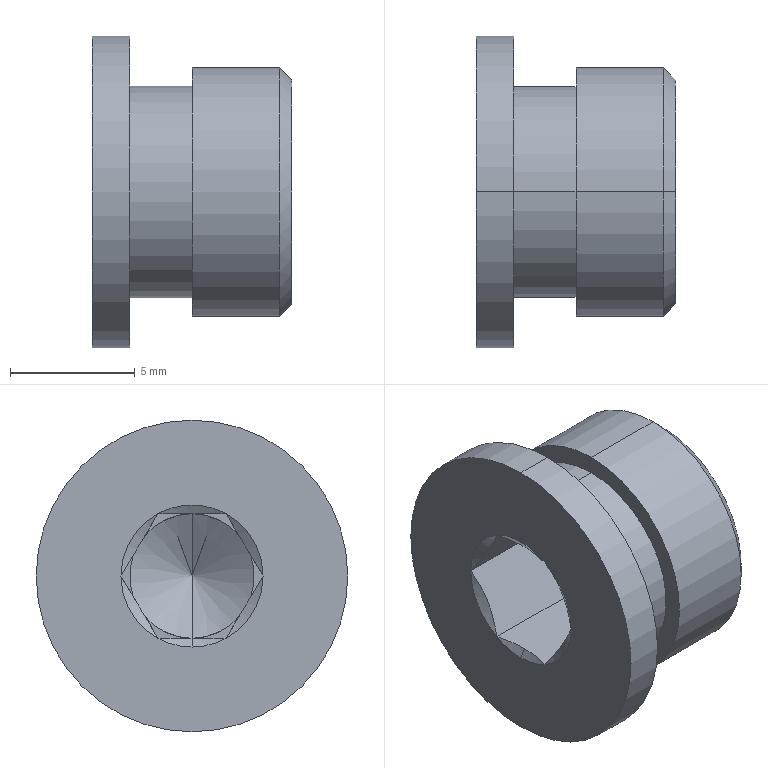Part | SolidWorks | features BaseBody 1 | 1 solid | 39 faces | box 8 x 12.5 x 12.5 mm | volume 511.919 mm3 | plane 20 | cone 11 | cylinder 8 | commonest cylinder face diameters 5 x2 8.5 x2 10 x2 12.5 x2
STEP:
#1=CARTESIAN_POINT('',(9.1,110.5,31.));
#2=VERTEX_POINT('',#1);
#3=CARTESIAN_POINT('',(9.1,110.5,22.));
#4=VERTEX_POINT('',#3);
#5=CARTESIAN_POINT('',(9.1,110.5,26.5));
#6=DIRECTION('',(1.,0.,0.));
#7=DIRECTION('',(0.,0.,1.));
#8=AXIS2_PLACEMENT_3D('',#5,#6,#7);
#9=CIRCLE('',#8,4.5);
#10=EDGE_CURVE('',#2,#4,#9,.T.);
#11=ORIENTED_EDGE('',*,*,#10,.F.);
#12=CARTESIAN_POINT('',(8.6,110.5,31.5));
#13=VERTEX_POINT('',#12);
#14=CARTESIAN_POINT('',(9.1,110.5,31.));
#15=DIRECTION('',(-0.7071,0.,0.7071));
#16=VECTOR('',#15,1000.);
#17=LINE('',#14,#16);
#18=EDGE_CURVE('',#2,#13,#17,.T.);
#19=ORIENTED_EDGE('',*,*,#18,.T.);
#20=CARTESIAN_POINT('',(8.6,110.5,21.5));
#21=VERTEX_POINT('',#20);
#22=CARTESIAN_POINT('',(8.6,110.5,26.5));
#23=DIRECTION('',(-1.,0.,0.));
#24=DIRECTION('',(0.,0.,1.));
#25=AXIS2_PLACEMENT_3D('',#22,#23,#24);
#26=CIRCLE('',#25,5.);
#27=EDGE_CURVE('',#21,#13,#26,.T.);
#28=ORIENTED_EDGE('',*,*,#27,.F.);
#29=CARTESIAN_POINT('',(9.1,110.5,22.));
#30=DIRECTION('',(-0.7071,0.,-0.7071));
#31=VECTOR('',#30,1000.);
#32=LINE('',#29,#31);
#33=EDGE_CURVE('',#4,#21,#32,.T.);
#34=ORIENTED_EDGE('',*,*,#33,.F.);
#35=EDGE_LOOP('',(#11,#19,#28,#34));
#36=FACE_OUTER_BOUND('',#35,.T.);
#37=CARTESIAN_POINT('',(9.1,110.5,26.5));
#38=DIRECTION('',(-1.,0.,0.));
#39=DIRECTION('',(0.,0.,-1.));
#40=AXIS2_PLACEMENT_3D('',#37,#38,#39);
#41=CONICAL_SURFACE('',#40,4.5,0.7854);
#42=ADVANCED_FACE('',(#36),#41,.T.);
#43=CARTESIAN_POINT('',(8.043,110.5,26.5));
#44=VERTEX_POINT('',#43);
#45=CARTESIAN_POINT('',(6.6,110.5,24.));
#46=VERTEX_POINT('',#45);
#47=CARTESIAN_POINT('',(6.6,110.5,24.));
#48=DIRECTION('',(-0.5,0.,-0.866));
#49=VECTOR('',#48,1000.);
#50=LINE('',#47,#49);
#51=EDGE_CURVE('',#44,#46,#50,.T.);
#52=ORIENTED_EDGE('',*,*,#51,.F.);
#53=CARTESIAN_POINT('',(6.6,110.5,29.));
#54=VERTEX_POINT('',#53);
#55=CARTESIAN_POINT('',(6.6,110.5,29.));
#56=DIRECTION('',(-0.5,0.,0.866));
#57=VECTOR('',#56,1000.);
#58=LINE('',#55,#57);
#59=EDGE_CURVE('',#44,#54,#58,.T.);
#60=ORIENTED_EDGE('',*,*,#59,.T.);
#61=CARTESIAN_POINT('',(6.6,110.5,26.5));
#62=DIRECTION('',(-1.,0.,0.));
#63=DIRECTION('',(0.,0.,-1.));
#64=AXIS2_PLACEMENT_3D('',#61,#62,#63);
#65=CIRCLE('',#64,2.5);
#66=EDGE_CURVE('',#54,#46,#65,.T.);
#67=ORIENTED_EDGE('',*,*,#66,.T.);
#68=EDGE_LOOP('',(#52,#60,#67));
#69=FACE_OUTER_BOUND('',#68,.T.);
#70=CARTESIAN_POINT('',(6.6,110.5,26.5));
#71=DIRECTION('',(-1.,0.,0.));
#72=DIRECTION('',(0.,0.,-1.));
#73=AXIS2_PLACEMENT_3D('',#70,#71,#72);
#74=CONICAL_SURFACE('',#73,2.5,1.047);
#75=ADVANCED_FACE('',(#69),#74,.F.);
#76=ORIENTED_EDGE('',*,*,#66,.F.);
#77=CARTESIAN_POINT('',(5.6,110.5,29.));
#78=VERTEX_POINT('',#77);
#79=CARTESIAN_POINT('',(22.671,110.5,29.));
#80=DIRECTION('',(-1.,0.,0.));
#81=VECTOR('',#80,1000.);
#82=LINE('',#79,#81);
#83=EDGE_CURVE('',#54,#78,#82,.T.);
#84=ORIENTED_EDGE('',*,*,#83,.T.);
#85=CARTESIAN_POINT('',(5.6,112.36,28.17));
#86=VERTEX_POINT('',#85);
#87=CARTESIAN_POINT('',(5.6,110.5,26.5));
#88=DIRECTION('',(1.,0.,0.));
#89=DIRECTION('',(0.,0.,1.));
#90=AXIS2_PLACEMENT_3D('',#87,#88,#89);
#91=CIRCLE('',#90,2.5);
#92=EDGE_CURVE('',#86,#78,#91,.T.);
#93=ORIENTED_EDGE('',*,*,#92,.F.);
#94=CARTESIAN_POINT('',(5.6,112.858,27.33));
#95=VERTEX_POINT('',#94);
#96=CARTESIAN_POINT('',(5.6,110.5,26.5));
#97=DIRECTION('',(-1.,0.,0.));
#98=DIRECTION('',(0.,0.,-1.));
#99=AXIS2_PLACEMENT_3D('',#96,#97,#98);
#100=CIRCLE('',#99,2.5);
#101=EDGE_CURVE('',#86,#95,#100,.T.);
#102=ORIENTED_EDGE('',*,*,#101,.T.);
#103=CARTESIAN_POINT('',(5.6,112.858,25.67));
#104=VERTEX_POINT('',#103);
#105=CARTESIAN_POINT('',(5.6,110.5,26.5));
#106=DIRECTION('',(1.,0.,0.));
#107=DIRECTION('',(0.,0.,1.));
#108=AXIS2_PLACEMENT_3D('',#105,#106,#107);
#109=CIRCLE('',#108,2.5);
#110=EDGE_CURVE('',#104,#95,#109,.T.);
#111=ORIENTED_EDGE('',*,*,#110,.F.);
#112=CARTESIAN_POINT('',(5.6,112.36,24.83));
#113=VERTEX_POINT('',#112);
#114=CARTESIAN_POINT('',(5.6,110.5,26.5));
#115=DIRECTION('',(-1.,0.,0.));
#116=DIRECTION('',(0.,0.,-1.));
#117=AXIS2_PLACEMENT_3D('',#114,#115,#116);
#118=CIRCLE('',#117,2.5);
#119=EDGE_CURVE('',#104,#113,#118,.T.);
#120=ORIENTED_EDGE('',*,*,#119,.T.);
#121=CARTESIAN_POINT('',(5.6,110.5,24.));
#122=VERTEX_POINT('',#121);
#123=CARTESIAN_POINT('',(5.6,110.5,26.5));
#124=DIRECTION('',(1.,0.,0.));
#125=DIRECTION('',(0.,0.,1.));
#126=AXIS2_PLACEMENT_3D('',#123,#124,#125);
#127=CIRCLE('',#126,2.5);
#128=EDGE_CURVE('',#122,#113,#127,.T.);
#129=ORIENTED_EDGE('',*,*,#128,.F.);
#130=CARTESIAN_POINT('',(22.671,110.5,24.));
#131=DIRECTION('',(-1.,0.,0.));
#132=VECTOR('',#131,1000.);
#133=LINE('',#130,#132);
#134=EDGE_CURVE('',#46,#122,#133,.T.);
#135=ORIENTED_EDGE('',*,*,#134,.F.);
#136=EDGE_LOOP('',(#76,#84,#93,#102,#111,#120,#129,#135));
#137=FACE_OUTER_BOUND('',#136,.T.);
#138=CARTESIAN_POINT('',(22.671,110.5,26.5));
#139=DIRECTION('',(-1.,0.,0.));
#140=DIRECTION('',(0.,0.,-1.));
#141=AXIS2_PLACEMENT_3D('',#138,#139,#140);
#142=CYLINDRICAL_SURFACE('',#141,2.5);
#143=ADVANCED_FACE('',(#137),#142,.F.);
#144=CARTESIAN_POINT('',(1.1,109.132,24.));
#145=VERTEX_POINT('',#144);
#146=CARTESIAN_POINT('',(1.302,110.5,24.));
#147=VERTEX_POINT('',#146);
#148=CARTESIAN_POINT('',(1.1,109.132,24.));
#149=CARTESIAN_POINT('',(1.161,109.353,24.));
#150=CARTESIAN_POINT('',(1.212,109.578,24.));
#151=CARTESIAN_POINT('',(1.283,110.036,24.));
#152=CARTESIAN_POINT('',(1.302,110.269,24.));
#153=CARTESIAN_POINT('',(1.302,110.5,24.));
#154=B_SPLINE_CURVE_WITH_KNOTS('',3,(#148,#149,#150,#151,#152,#153),.UNSPECIFIED.,.F.,.F.,(4,2,4),(0.001327,0.002017,0.002707),.UNSPECIFIED.);
#155=EDGE_CURVE('',#145,#147,#154,.T.);
#156=ORIENTED_EDGE('',*,*,#155,.T.);
#157=CARTESIAN_POINT('',(1.1,110.5,23.65));
#158=VERTEX_POINT('',#157);
#159=CARTESIAN_POINT('',(1.1,110.5,23.65));
#160=DIRECTION('',(-0.5,0.,-0.866));
#161=VECTOR('',#160,1000.);
#162=LINE('',#159,#161);
#163=EDGE_CURVE('',#147,#158,#162,.T.);
#164=ORIENTED_EDGE('',*,*,#163,.T.);
#165=CARTESIAN_POINT('',(1.1,110.5,26.5));
#166=DIRECTION('',(-1.,0.,0.));
#167=DIRECTION('',(0.,0.,-1.));
#168=AXIS2_PLACEMENT_3D('',#165,#166,#167);
#169=CIRCLE('',#168,2.85);
#170=EDGE_CURVE('',#158,#145,#169,.T.);
#171=ORIENTED_EDGE('',*,*,#170,.T.);
#172=EDGE_LOOP('',(#156,#164,#171));
#173=FACE_OUTER_BOUND('',#172,.T.);
#174=CARTESIAN_POINT('',(1.1,110.5,26.5));
#175=DIRECTION('',(-1.,0.,0.));
#176=DIRECTION('',(0.,0.,-1.));
#177=AXIS2_PLACEMENT_3D('',#174,#175,#176);
#178=CONICAL_SURFACE('',#177,2.85,1.047);
#179=ADVANCED_FACE('',(#173),#178,.F.);
#180=ORIENTED_EDGE('',*,*,#27,.T.);
#181=CARTESIAN_POINT('',(5.1,110.5,31.5));
#182=VERTEX_POINT('',#181);
#183=CARTESIAN_POINT('',(31.242,110.5,31.5));
#184=DIRECTION('',(-1.,0.,0.));
#185=VECTOR('',#184,1000.);
#186=LINE('',#183,#185);
#187=EDGE_CURVE('',#13,#182,#186,.T.);
#188=ORIENTED_EDGE('',*,*,#187,.T.);
#189=CARTESIAN_POINT('',(5.1,110.5,21.5));
#190=VERTEX_POINT('',#189);
#191=CARTESIAN_POINT('',(5.1,110.5,26.5));
#192=DIRECTION('',(1.,0.,0.));
#193=DIRECTION('',(0.,0.,1.));
#194=AXIS2_PLACEMENT_3D('',#191,#192,#193);
#195=CIRCLE('',#194,5.);
#196=EDGE_CURVE('',#182,#190,#195,.T.);
#197=ORIENTED_EDGE('',*,*,#196,.T.);
#198=CARTESIAN_POINT('',(31.242,110.5,21.5));
#199=DIRECTION('',(-1.,0.,0.));
#200=VECTOR('',#199,1000.);
#201=LINE('',#198,#200);
#202=EDGE_CURVE('',#21,#190,#201,.T.);
#203=ORIENTED_EDGE('',*,*,#202,.F.);
#204=EDGE_LOOP('',(#180,#188,#197,#203));
#205=FACE_OUTER_BOUND('',#204,.T.);
#206=CARTESIAN_POINT('',(31.242,110.5,26.5));
#207=DIRECTION('',(-1.,0.,0.));
#208=DIRECTION('',(0.,0.,-1.));
#209=AXIS2_PLACEMENT_3D('',#206,#207,#208);
#210=CYLINDRICAL_SURFACE('',#209,5.);
#211=ADVANCED_FACE('',(#205),#210,.T.);
#212=CARTESIAN_POINT('',(5.1,110.5,30.75));
#213=VERTEX_POINT('',#212);
#214=CARTESIAN_POINT('',(5.1,110.5,22.25));
#215=VERTEX_POINT('',#214);
#216=CARTESIAN_POINT('',(5.1,110.5,26.5));
#217=DIRECTION('',(1.,0.,0.));
#218=DIRECTION('',(0.,0.,1.));
#219=AXIS2_PLACEMENT_3D('',#216,#217,#218);
#220=CIRCLE('',#219,4.25);
#221=EDGE_CURVE('',#213,#215,#220,.T.);
#222=ORIENTED_EDGE('',*,*,#221,.F.);
#223=CARTESIAN_POINT('',(2.6,110.5,30.75));
#224=VERTEX_POINT('',#223);
#225=CARTESIAN_POINT('',(5.1,110.5,30.75));
#226=DIRECTION('',(-1.,0.,0.));
#227=VECTOR('',#226,1000.);
#228=LINE('',#225,#227);
#229=EDGE_CURVE('',#213,#224,#228,.T.);
#230=ORIENTED_EDGE('',*,*,#229,.T.);
#231=CARTESIAN_POINT('',(2.6,110.5,22.25));
#232=VERTEX_POINT('',#231);
#233=CARTESIAN_POINT('',(2.6,110.5,26.5));
#234=DIRECTION('',(1.,0.,0.));
#235=DIRECTION('',(0.,0.,1.));
#236=AXIS2_PLACEMENT_3D('',#233,#234,#235);
#237=CIRCLE('',#236,4.25);
#238=EDGE_CURVE('',#224,#232,#237,.T.);
#239=ORIENTED_EDGE('',*,*,#238,.T.);
#240=CARTESIAN_POINT('',(5.1,110.5,22.25));
#241=DIRECTION('',(-1.,0.,0.));
#242=VECTOR('',#241,1000.);
#243=LINE('',#240,#242);
#244=EDGE_CURVE('',#215,#232,#243,.T.);
#245=ORIENTED_EDGE('',*,*,#244,.F.);
#246=EDGE_LOOP('',(#222,#230,#239,#245));
#247=FACE_OUTER_BOUND('',#246,.T.);
#248=CARTESIAN_POINT('',(5.1,110.5,26.5));
#249=DIRECTION('',(-1.,0.,0.));
#250=DIRECTION('',(0.,0.,-1.));
#251=AXIS2_PLACEMENT_3D('',#248,#249,#250);
#252=CYLINDRICAL_SURFACE('',#251,4.25);
#253=ADVANCED_FACE('',(#247),#252,.T.);
#254=CARTESIAN_POINT('',(2.6,110.5,32.75));
#255=VERTEX_POINT('',#254);
#256=CARTESIAN_POINT('',(2.6,110.5,20.25));
#257=VERTEX_POINT('',#256);
#258=CARTESIAN_POINT('',(2.6,110.5,26.5));
#259=DIRECTION('',(1.,0.,0.));
#260=DIRECTION('',(0.,0.,1.));
#261=AXIS2_PLACEMENT_3D('',#258,#259,#260);
#262=CIRCLE('',#261,6.25);
#263=EDGE_CURVE('',#255,#257,#262,.T.);
#264=ORIENTED_EDGE('',*,*,#263,.F.);
#265=CARTESIAN_POINT('',(1.1,110.5,32.75));
#266=VERTEX_POINT('',#265);
#267=CARTESIAN_POINT('',(2.6,110.5,32.75));
#268=DIRECTION('',(-1.,0.,0.));
#269=VECTOR('',#268,1000.);
#270=LINE('',#267,#269);
#271=EDGE_CURVE('',#255,#266,#270,.T.);
#272=ORIENTED_EDGE('',*,*,#271,.T.);
#273=CARTESIAN_POINT('',(1.1,110.5,20.25));
#274=VERTEX_POINT('',#273);
#275=CARTESIAN_POINT('',(1.1,110.5,26.5));
#276=DIRECTION('',(1.,0.,0.));
#277=DIRECTION('',(0.,0.,1.));
#278=AXIS2_PLACEMENT_3D('',#275,#276,#277);
#279=CIRCLE('',#278,6.25);
#280=EDGE_CURVE('',#266,#274,#279,.T.);
#281=ORIENTED_EDGE('',*,*,#280,.T.);
#282=CARTESIAN_POINT('',(2.6,110.5,20.25));
#283=DIRECTION('',(-1.,0.,0.));
#284=VECTOR('',#283,1000.);
#285=LINE('',#282,#284);
#286=EDGE_CURVE('',#257,#274,#285,.T.);
#287=ORIENTED_EDGE('',*,*,#286,.F.);
#288=EDGE_LOOP('',(#264,#272,#281,#287));
#289=FACE_OUTER_BOUND('',#288,.T.);
#290=CARTESIAN_POINT('',(2.6,110.5,26.5));
#291=DIRECTION('',(-1.,0.,0.));
#292=DIRECTION('',(0.,0.,-1.));
#293=AXIS2_PLACEMENT_3D('',#290,#291,#292);
#294=CYLINDRICAL_SURFACE('',#293,6.25);
#295=ADVANCED_FACE('',(#289),#294,.T.);
#296=CARTESIAN_POINT('',(5.6,107.65,26.5));
#297=VERTEX_POINT('',#296);
#298=CARTESIAN_POINT('',(5.6,108.142,27.33));
#299=VERTEX_POINT('',#298);
#300=CARTESIAN_POINT('',(5.6,107.65,26.5));
#301=DIRECTION('',(0.,0.5098,0.8603));
#302=VECTOR('',#301,1000.);
#303=LINE('',#300,#302);
#304=EDGE_CURVE('',#297,#299,#303,.T.);
#305=ORIENTED_EDGE('',*,*,#304,.T.);
#306=CARTESIAN_POINT('',(5.6,108.142,25.67));
#307=VERTEX_POINT('',#306);
#308=CARTESIAN_POINT('',(5.6,110.5,26.5));
#309=DIRECTION('',(1.,0.,0.));
#310=DIRECTION('',(0.,0.,1.));
#311=AXIS2_PLACEMENT_3D('',#308,#309,#310);
#312=CIRCLE('',#311,2.5);
#313=EDGE_CURVE('',#299,#307,#312,.T.);
#314=ORIENTED_EDGE('',*,*,#313,.T.);
#315=CARTESIAN_POINT('',(5.6,107.65,26.5));
#316=DIRECTION('',(0.,-0.5098,0.8603));
#317=VECTOR('',#316,1000.);
#318=LINE('',#315,#317);
#319=EDGE_CURVE('',#307,#297,#318,.T.);
#320=ORIENTED_EDGE('',*,*,#319,.T.);
#321=EDGE_LOOP('',(#305,#314,#320));
#322=FACE_OUTER_BOUND('',#321,.T.);
#323=CARTESIAN_POINT('',(5.6,110.5,31.309));
#324=DIRECTION('',(1.,0.,0.));
#325=DIRECTION('',(0.,0.,1.));
#326=AXIS2_PLACEMENT_3D('',#323,#324,#325);
#327=PLANE('',#326);
#328=ADVANCED_FACE('',(#322),#327,.F.);
#329=CARTESIAN_POINT('',(5.6,109.132,24.));
#330=VERTEX_POINT('',#329);
#331=CARTESIAN_POINT('',(5.6,108.64,24.83));
#332=VERTEX_POINT('',#331);
#333=CARTESIAN_POINT('',(5.6,107.65,26.5));
#334=DIRECTION('',(0.,-0.5098,0.8603));
#335=VECTOR('',#334,1000.);
#336=LINE('',#333,#335);
#337=EDGE_CURVE('',#330,#332,#336,.T.);
#338=ORIENTED_EDGE('',*,*,#337,.T.);
#339=CARTESIAN_POINT('',(5.6,110.5,26.5));
#340=DIRECTION('',(-1.,0.,0.));
#341=DIRECTION('',(0.,0.,-1.));
#342=AXIS2_PLACEMENT_3D('',#339,#340,#341);
#343=CIRCLE('',#342,2.5);
#344=EDGE_CURVE('',#122,#332,#343,.T.);
#345=ORIENTED_EDGE('',*,*,#344,.F.);
#346=CARTESIAN_POINT('',(5.6,109.132,24.));
#347=DIRECTION('',(0.,-1.,0.));
#348=VECTOR('',#347,1000.);
#349=LINE('',#346,#348);
#350=EDGE_CURVE('',#122,#330,#349,.T.);
#351=ORIENTED_EDGE('',*,*,#350,.T.);
#352=EDGE_LOOP('',(#338,#345,#351));
#353=FACE_OUTER_BOUND('',#352,.T.);
#354=CARTESIAN_POINT('',(5.6,110.5,31.309));
#355=DIRECTION('',(1.,0.,0.));
#356=DIRECTION('',(0.,0.,1.));
#357=AXIS2_PLACEMENT_3D('',#354,#355,#356);
#358=PLANE('',#357);
#359=ADVANCED_FACE('',(#353),#358,.F.);
#360=CARTESIAN_POINT('',(5.6,111.868,24.));
#361=VERTEX_POINT('',#360);
#362=CARTESIAN_POINT('',(5.6,109.132,24.));
#363=DIRECTION('',(0.,-1.,0.));
#364=VECTOR('',#363,1000.);
#365=LINE('',#362,#364);
#366=EDGE_CURVE('',#361,#122,#365,.T.);
#367=ORIENTED_EDGE('',*,*,#366,.T.);
#368=ORIENTED_EDGE('',*,*,#128,.T.);
#369=CARTESIAN_POINT('',(5.6,113.35,26.5));
#370=DIRECTION('',(0.,-0.5098,-0.8603));
#371=VECTOR('',#370,1000.);
#372=LINE('',#369,#371);
#373=EDGE_CURVE('',#113,#361,#372,.T.);
#374=ORIENTED_EDGE('',*,*,#373,.T.);
#375=EDGE_LOOP('',(#367,#368,#374));
#376=FACE_OUTER_BOUND('',#375,.T.);
#377=CARTESIAN_POINT('',(5.6,110.5,31.309));
#378=DIRECTION('',(1.,0.,0.));
#379=DIRECTION('',(0.,0.,1.));
#380=AXIS2_PLACEMENT_3D('',#377,#378,#379);
#381=PLANE('',#380);
#382=ADVANCED_FACE('',(#376),#381,.F.);
#383=CARTESIAN_POINT('',(5.6,113.35,26.5));
#384=VERTEX_POINT('',#383);
#385=CARTESIAN_POINT('',(5.6,113.35,26.5));
#386=DIRECTION('',(0.,-0.5098,-0.8603));
#387=VECTOR('',#386,1000.);
#388=LINE('',#385,#387);
#389=EDGE_CURVE('',#384,#104,#388,.T.);
#390=ORIENTED_EDGE('',*,*,#389,.T.);
#391=ORIENTED_EDGE('',*,*,#110,.T.);
#392=CARTESIAN_POINT('',(5.6,113.35,26.5));
#393=DIRECTION('',(0.,0.5098,-0.8603));
#394=VECTOR('',#393,1000.);
#395=LINE('',#392,#394);
#396=EDGE_CURVE('',#95,#384,#395,.T.);
#397=ORIENTED_EDGE('',*,*,#396,.T.);
#398=EDGE_LOOP('',(#390,#391,#397));
#399=FACE_OUTER_BOUND('',#398,.T.);
#400=CARTESIAN_POINT('',(5.6,110.5,31.309));
#401=DIRECTION('',(1.,0.,0.));
#402=DIRECTION('',(0.,0.,1.));
#403=AXIS2_PLACEMENT_3D('',#400,#401,#402);
#404=PLANE('',#403);
#405=ADVANCED_FACE('',(#399),#404,.F.);
#406=CARTESIAN_POINT('',(5.6,109.132,29.));
#407=VERTEX_POINT('',#406);
#408=CARTESIAN_POINT('',(5.6,109.132,29.));
#409=DIRECTION('',(0.,1.,0.));
#410=VECTOR('',#409,1000.);
#411=LINE('',#408,#410);
#412=EDGE_CURVE('',#407,#78,#411,.T.);
#413=ORIENTED_EDGE('',*,*,#412,.T.);
#414=CARTESIAN_POINT('',(5.6,108.64,28.17));
#415=VERTEX_POINT('',#414);
#416=CARTESIAN_POINT('',(5.6,110.5,26.5));
#417=DIRECTION('',(1.,0.,0.));
#418=DIRECTION('',(0.,0.,1.));
#419=AXIS2_PLACEMENT_3D('',#416,#417,#418);
#420=CIRCLE('',#419,2.5);
#421=EDGE_CURVE('',#78,#415,#420,.T.);
#422=ORIENTED_EDGE('',*,*,#421,.T.);
#423=CARTESIAN_POINT('',(5.6,107.65,26.5));
#424=DIRECTION('',(0.,0.5098,0.8603));
#425=VECTOR('',#424,1000.);
#426=LINE('',#423,#425);
#427=EDGE_CURVE('',#415,#407,#426,.T.);
#428=ORIENTED_EDGE('',*,*,#427,.T.);
#429=EDGE_LOOP('',(#413,#422,#428));
#430=FACE_OUTER_BOUND('',#429,.T.);
#431=CARTESIAN_POINT('',(5.6,110.5,31.309));
#432=DIRECTION('',(1.,0.,0.));
#433=DIRECTION('',(0.,0.,1.));
#434=AXIS2_PLACEMENT_3D('',#431,#432,#433);
#435=PLANE('',#434);
#436=ADVANCED_FACE('',(#430),#435,.F.);
#437=CARTESIAN_POINT('',(2.6,110.5,26.5));
#438=DIRECTION('',(1.,0.,0.));
#439=DIRECTION('',(0.,0.,1.));
#440=AXIS2_PLACEMENT_3D('',#437,#438,#439);
#441=CIRCLE('',#440,6.25);
#442=EDGE_CURVE('',#257,#255,#441,.T.);
#443=ORIENTED_EDGE('',*,*,#442,.T.);
#444=ORIENTED_EDGE('',*,*,#263,.T.);
#445=EDGE_LOOP('',(#443,#444));
#446=FACE_OUTER_BOUND('',#445,.T.);
#447=CARTESIAN_POINT('',(2.6,110.5,26.5));
#448=DIRECTION('',(1.,0.,0.));
#449=DIRECTION('',(0.,0.,1.));
#450=AXIS2_PLACEMENT_3D('',#447,#448,#449);
#451=CIRCLE('',#450,4.25);
#452=EDGE_CURVE('',#232,#224,#451,.T.);
#453=ORIENTED_EDGE('',*,*,#452,.F.);
#454=ORIENTED_EDGE('',*,*,#238,.F.);
#455=EDGE_LOOP('',(#453,#454));
#456=FACE_BOUND('',#455,.T.);
#457=CARTESIAN_POINT('',(2.6,110.5,26.5));
#458=DIRECTION('',(1.,0.,0.));
#459=DIRECTION('',(0.,0.,1.));
#460=AXIS2_PLACEMENT_3D('',#457,#458,#459);
#461=PLANE('',#460);
#462=ADVANCED_FACE('',(#446,#456),#461,.T.);
#463=ORIENTED_EDGE('',*,*,#271,.F.);
#464=ORIENTED_EDGE('',*,*,#442,.F.);
#465=ORIENTED_EDGE('',*,*,#286,.T.);
#466=CARTESIAN_POINT('',(1.1,110.5,26.5));
#467=DIRECTION('',(1.,0.,0.));
#468=DIRECTION('',(0.,0.,1.));
#469=AXIS2_PLACEMENT_3D('',#466,#467,#468);
#470=CIRCLE('',#469,6.25);
#471=EDGE_CURVE('',#274,#266,#470,.T.);
#472=ORIENTED_EDGE('',*,*,#471,.T.);
#473=EDGE_LOOP('',(#463,#464,#465,#472));
#474=FACE_OUTER_BOUND('',#473,.T.);
#475=CARTESIAN_POINT('',(2.6,110.5,26.5));
#476=DIRECTION('',(-1.,0.,0.));
#477=DIRECTION('',(0.,0.,-1.));
#478=AXIS2_PLACEMENT_3D('',#475,#476,#477);
#479=CYLINDRICAL_SURFACE('',#478,6.25);
#480=ADVANCED_FACE('',(#474),#479,.T.);
#481=CARTESIAN_POINT('',(1.1,109.132,29.));
#482=VERTEX_POINT('',#481);
#483=CARTESIAN_POINT('',(1.1,111.868,29.));
#484=VERTEX_POINT('',#483);
#485=CARTESIAN_POINT('',(1.1,110.5,26.5));
#486=DIRECTION('',(-1.,0.,0.));
#487=DIRECTION('',(0.,0.,-1.));
#488=AXIS2_PLACEMENT_3D('',#485,#486,#487);
#489=CIRCLE('',#488,2.85);
#490=EDGE_CURVE('',#482,#484,#489,.T.);
#491=ORIENTED_EDGE('',*,*,#490,.F.);
#492=CARTESIAN_POINT('',(1.1,107.65,26.5));
#493=VERTEX_POINT('',#492);
#494=CARTESIAN_POINT('',(1.1,110.5,26.5));
#495=DIRECTION('',(-1.,0.,0.));
#496=DIRECTION('',(0.,0.,-1.));
#497=AXIS2_PLACEMENT_3D('',#494,#495,#496);
#498=CIRCLE('',#497,2.85);
#499=EDGE_CURVE('',#493,#482,#498,.T.);
#500=ORIENTED_EDGE('',*,*,#499,.F.);
#501=CARTESIAN_POINT('',(1.1,110.5,26.5));
#502=DIRECTION('',(-1.,0.,0.));
#503=DIRECTION('',(0.,0.,-1.));
#504=AXIS2_PLACEMENT_3D('',#501,#502,#503);
#505=CIRCLE('',#504,2.85);
#506=EDGE_CURVE('',#145,#493,#505,.T.);
#507=ORIENTED_EDGE('',*,*,#506,.F.);
#508=ORIENTED_EDGE('',*,*,#170,.F.);
#509=CARTESIAN_POINT('',(1.1,111.868,24.));
#510=VERTEX_POINT('',#509);
#511=CARTESIAN_POINT('',(1.1,110.5,26.5));
#512=DIRECTION('',(-1.,0.,0.));
#513=DIRECTION('',(0.,0.,-1.));
#514=AXIS2_PLACEMENT_3D('',#511,#512,#513);
#515=CIRCLE('',#514,2.85);
#516=EDGE_CURVE('',#510,#158,#515,.T.);
#517=ORIENTED_EDGE('',*,*,#516,.F.);
#518=CARTESIAN_POINT('',(1.1,113.35,26.5));
#519=VERTEX_POINT('',#518);
#520=CARTESIAN_POINT('',(1.1,110.5,26.5));
#521=DIRECTION('',(-1.,0.,0.));
#522=DIRECTION('',(0.,0.,-1.));
#523=AXIS2_PLACEMENT_3D('',#520,#521,#522);
#524=CIRCLE('',#523,2.85);
#525=EDGE_CURVE('',#519,#510,#524,.T.);
#526=ORIENTED_EDGE('',*,*,#525,.F.);
#527=CARTESIAN_POINT('',(1.1,110.5,26.5));
#528=DIRECTION('',(-1.,0.,0.));
#529=DIRECTION('',(0.,0.,-1.));
#530=AXIS2_PLACEMENT_3D('',#527,#528,#529);
#531=CIRCLE('',#530,2.85);
#532=EDGE_CURVE('',#484,#519,#531,.T.);
#533=ORIENTED_EDGE('',*,*,#532,.F.);
#534=EDGE_LOOP('',(#491,#500,#507,#508,#517,#526,#533));
#535=FACE_BOUND('',#534,.T.);
#536=ORIENTED_EDGE('',*,*,#471,.F.);
#537=ORIENTED_EDGE('',*,*,#280,.F.);
#538=EDGE_LOOP('',(#536,#537));
#539=FACE_OUTER_BOUND('',#538,.T.);
#540=CARTESIAN_POINT('',(1.1,110.5,26.5));
#541=DIRECTION('',(1.,0.,0.));
#542=DIRECTION('',(0.,0.,1.));
#543=AXIS2_PLACEMENT_3D('',#540,#541,#542);
#544=PLANE('',#543);
#545=ADVANCED_FACE('',(#535,#539),#544,.F.);
#546=ORIENTED_EDGE('',*,*,#229,.F.);
#547=CARTESIAN_POINT('',(5.1,110.5,26.5));
#548=DIRECTION('',(1.,0.,0.));
#549=DIRECTION('',(0.,0.,1.));
#550=AXIS2_PLACEMENT_3D('',#547,#548,#549);
#551=CIRCLE('',#550,4.25);
#552=EDGE_CURVE('',#215,#213,#551,.T.);
#553=ORIENTED_EDGE('',*,*,#552,.F.);
#554=ORIENTED_EDGE('',*,*,#244,.T.);
#555=ORIENTED_EDGE('',*,*,#452,.T.);
#556=EDGE_LOOP('',(#546,#553,#554,#555));
#557=FACE_OUTER_BOUND('',#556,.T.);
#558=CARTESIAN_POINT('',(5.1,110.5,26.5));
#559=DIRECTION('',(-1.,0.,0.));
#560=DIRECTION('',(0.,0.,-1.));
#561=AXIS2_PLACEMENT_3D('',#558,#559,#560);
#562=CYLINDRICAL_SURFACE('',#561,4.25);
#563=ADVANCED_FACE('',(#557),#562,.T.);
#564=CARTESIAN_POINT('',(5.1,110.5,26.5));
#565=DIRECTION('',(1.,0.,0.));
#566=DIRECTION('',(0.,0.,1.));
#567=AXIS2_PLACEMENT_3D('',#564,#565,#566);
#568=CIRCLE('',#567,5.);
#569=EDGE_CURVE('',#190,#182,#568,.T.);
#570=ORIENTED_EDGE('',*,*,#569,.F.);
#571=ORIENTED_EDGE('',*,*,#196,.F.);
#572=EDGE_LOOP('',(#570,#571));
#573=FACE_OUTER_BOUND('',#572,.T.);
#574=ORIENTED_EDGE('',*,*,#552,.T.);
#575=ORIENTED_EDGE('',*,*,#221,.T.);
#576=EDGE_LOOP('',(#574,#575));
#577=FACE_BOUND('',#576,.T.);
#578=CARTESIAN_POINT('',(5.1,110.5,26.5));
#579=DIRECTION('',(1.,0.,0.));
#580=DIRECTION('',(0.,0.,1.));
#581=AXIS2_PLACEMENT_3D('',#578,#579,#580);
#582=PLANE('',#581);
#583=ADVANCED_FACE('',(#573,#577),#582,.F.);
#584=ORIENTED_EDGE('',*,*,#187,.F.);
#585=CARTESIAN_POINT('',(8.6,110.5,26.5));
#586=DIRECTION('',(-1.,0.,0.));
#587=DIRECTION('',(0.,0.,1.));
#588=AXIS2_PLACEMENT_3D('',#585,#586,#587);
#589=CIRCLE('',#588,5.);
#590=EDGE_CURVE('',#13,#21,#589,.T.);
#591=ORIENTED_EDGE('',*,*,#590,.T.);
#592=ORIENTED_EDGE('',*,*,#202,.T.);
#593=ORIENTED_EDGE('',*,*,#569,.T.);
#594=EDGE_LOOP('',(#584,#591,#592,#593));
#595=FACE_OUTER_BOUND('',#594,.T.);
#596=CARTESIAN_POINT('',(31.242,110.5,26.5));
#597=DIRECTION('',(-1.,0.,0.));
#598=DIRECTION('',(0.,0.,-1.));
#599=AXIS2_PLACEMENT_3D('',#596,#597,#598);
#600=CYLINDRICAL_SURFACE('',#599,5.);
#601=ADVANCED_FACE('',(#595),#600,.T.);
#602=CARTESIAN_POINT('',(9.1,110.5,26.5));
#603=DIRECTION('',(1.,0.,0.));
#604=DIRECTION('',(0.,0.,1.));
#605=AXIS2_PLACEMENT_3D('',#602,#603,#604);
#606=CIRCLE('',#605,4.5);
#607=EDGE_CURVE('',#4,#2,#606,.T.);
#608=ORIENTED_EDGE('',*,*,#607,.T.);
#609=ORIENTED_EDGE('',*,*,#10,.T.);
#610=EDGE_LOOP('',(#608,#609));
#611=FACE_OUTER_BOUND('',#610,.T.);
#612=CARTESIAN_POINT('',(9.1,110.5,26.5));
#613=DIRECTION('',(1.,0.,0.));
#614=DIRECTION('',(0.,0.,1.));
#615=AXIS2_PLACEMENT_3D('',#612,#613,#614);
#616=PLANE('',#615);
#617=ADVANCED_FACE('',(#611),#616,.T.);
#618=CARTESIAN_POINT('',(5.6,107.65,26.5));
#619=DIRECTION('',(-1.,0.,0.));
#620=VECTOR('',#619,1000.);
#621=LINE('',#618,#620);
#622=EDGE_CURVE('',#297,#493,#621,.T.);
#623=ORIENTED_EDGE('',*,*,#622,.T.);
#624=CARTESIAN_POINT('',(1.1,109.132,29.));
#625=CARTESIAN_POINT('',(1.24,108.89,28.592));
#626=CARTESIAN_POINT('',(1.33,108.644,28.178));
#627=CARTESIAN_POINT('',(1.33,108.266,27.539));
#628=CARTESIAN_POINT('',(1.308,108.14,27.327));
#629=CARTESIAN_POINT('',(1.228,107.893,26.91));
#630=CARTESIAN_POINT('',(1.17,107.771,26.704));
#631=CARTESIAN_POINT('',(1.1,107.65,26.5));
#632=B_SPLINE_CURVE_WITH_KNOTS('',3,(#624,#625,#626,#627,#628,#629,#630,#631),.UNSPECIFIED.,.F.,.F.,(4,2,2,4),(0.00000024,0.001469,0.002204,0.002938),.UNSPECIFIED.);
#633=EDGE_CURVE('',#482,#493,#632,.T.);
#634=ORIENTED_EDGE('',*,*,#633,.F.);
#635=CARTESIAN_POINT('',(5.6,109.132,29.));
#636=DIRECTION('',(-1.,0.,0.));
#637=VECTOR('',#636,1000.);
#638=LINE('',#635,#637);
#639=EDGE_CURVE('',#407,#482,#638,.T.);
#640=ORIENTED_EDGE('',*,*,#639,.F.);
#641=ORIENTED_EDGE('',*,*,#427,.F.);
#642=CARTESIAN_POINT('',(5.6,107.65,26.5));
#643=DIRECTION('',(0.,0.5098,0.8603));
#644=VECTOR('',#643,1000.);
#645=LINE('',#642,#644);
#646=EDGE_CURVE('',#299,#415,#645,.T.);
#647=ORIENTED_EDGE('',*,*,#646,.F.);
#648=ORIENTED_EDGE('',*,*,#304,.F.);
#649=EDGE_LOOP('',(#623,#634,#640,#641,#647,#648));
#650=FACE_OUTER_BOUND('',#649,.T.);
#651=CARTESIAN_POINT('',(5.6,107.65,26.5));
#652=DIRECTION('',(0.,-0.8603,0.5098));
#653=DIRECTION('',(0.,-0.5098,-0.8603));
#654=AXIS2_PLACEMENT_3D('',#651,#652,#653);
#655=PLANE('',#654);
#656=ADVANCED_FACE('',(#650),#655,.F.);
#657=CARTESIAN_POINT('',(5.6,109.132,24.));
#658=DIRECTION('',(-1.,0.,0.));
#659=VECTOR('',#658,1000.);
#660=LINE('',#657,#659);
#661=EDGE_CURVE('',#330,#145,#660,.T.);
#662=ORIENTED_EDGE('',*,*,#661,.T.);
#663=CARTESIAN_POINT('',(1.1,107.65,26.5));
#664=CARTESIAN_POINT('',(1.24,107.892,26.092));
#665=CARTESIAN_POINT('',(1.33,108.137,25.678));
#666=CARTESIAN_POINT('',(1.33,108.516,25.039));
#667=CARTESIAN_POINT('',(1.308,108.642,24.827));
#668=CARTESIAN_POINT('',(1.228,108.889,24.41));
#669=CARTESIAN_POINT('',(1.17,109.011,24.204));
#670=CARTESIAN_POINT('',(1.1,109.132,24.));
#671=B_SPLINE_CURVE_WITH_KNOTS('',3,(#663,#664,#665,#666,#667,#668,#669,#670),.UNSPECIFIED.,.F.,.F.,(4,2,2,4),(0.00000024,0.001469,0.002204,0.002938),.UNSPECIFIED.);
#672=EDGE_CURVE('',#493,#145,#671,.T.);
#673=ORIENTED_EDGE('',*,*,#672,.F.);
#674=ORIENTED_EDGE('',*,*,#622,.F.);
#675=ORIENTED_EDGE('',*,*,#319,.F.);
#676=CARTESIAN_POINT('',(5.6,107.65,26.5));
#677=DIRECTION('',(0.,-0.5098,0.8603));
#678=VECTOR('',#677,1000.);
#679=LINE('',#676,#678);
#680=EDGE_CURVE('',#332,#307,#679,.T.);
#681=ORIENTED_EDGE('',*,*,#680,.F.);
#682=ORIENTED_EDGE('',*,*,#337,.F.);
#683=EDGE_LOOP('',(#662,#673,#674,#675,#681,#682));
#684=FACE_OUTER_BOUND('',#683,.T.);
#685=CARTESIAN_POINT('',(5.6,107.65,26.5));
#686=DIRECTION('',(0.,-0.8603,-0.5098));
#687=DIRECTION('',(0.,0.5098,-0.8603));
#688=AXIS2_PLACEMENT_3D('',#685,#686,#687);
#689=PLANE('',#688);
#690=ADVANCED_FACE('',(#684),#689,.F.);
#691=CARTESIAN_POINT('',(5.6,111.868,24.));
#692=DIRECTION('',(-1.,0.,0.));
#693=VECTOR('',#692,1000.);
#694=LINE('',#691,#693);
#695=EDGE_CURVE('',#361,#510,#694,.T.);
#696=ORIENTED_EDGE('',*,*,#695,.T.);
#697=CARTESIAN_POINT('',(1.302,110.5,24.));
#698=CARTESIAN_POINT('',(1.302,110.731,24.));
#699=CARTESIAN_POINT('',(1.283,110.96,24.));
#700=CARTESIAN_POINT('',(1.213,111.418,24.));
#701=CARTESIAN_POINT('',(1.162,111.646,24.));
#702=CARTESIAN_POINT('',(1.1,111.868,24.));
#703=B_SPLINE_CURVE_WITH_KNOTS('',3,(#697,#698,#699,#700,#701,#702),.UNSPECIFIED.,.F.,.F.,(4,2,4),(0.002707,0.003396,0.004086),.UNSPECIFIED.);
#704=EDGE_CURVE('',#147,#510,#703,.T.);
#705=ORIENTED_EDGE('',*,*,#704,.F.);
#706=ORIENTED_EDGE('',*,*,#155,.F.);
#707=ORIENTED_EDGE('',*,*,#661,.F.);
#708=ORIENTED_EDGE('',*,*,#350,.F.);
#709=ORIENTED_EDGE('',*,*,#366,.F.);
#710=EDGE_LOOP('',(#696,#705,#706,#707,#708,#709));
#711=FACE_OUTER_BOUND('',#710,.T.);
#712=CARTESIAN_POINT('',(5.6,109.132,24.));
#713=DIRECTION('',(0.,0.,-1.));
#714=DIRECTION('',(1.,0.,0.));
#715=AXIS2_PLACEMENT_3D('',#712,#713,#714);
#716=PLANE('',#715);
#717=ADVANCED_FACE('',(#711),#716,.F.);
#718=CARTESIAN_POINT('',(5.6,113.35,26.5));
#719=DIRECTION('',(-1.,0.,0.));
#720=VECTOR('',#719,1000.);
#721=LINE('',#718,#720);
#722=EDGE_CURVE('',#384,#519,#721,.T.);
#723=ORIENTED_EDGE('',*,*,#722,.T.);
#724=CARTESIAN_POINT('',(1.1,111.868,24.));
#725=CARTESIAN_POINT('',(1.24,112.11,24.408));
#726=CARTESIAN_POINT('',(1.33,112.356,24.822));
#727=CARTESIAN_POINT('',(1.33,112.734,25.461));
#728=CARTESIAN_POINT('',(1.308,112.86,25.673));
#729=CARTESIAN_POINT('',(1.228,113.107,26.09));
#730=CARTESIAN_POINT('',(1.17,113.229,26.296));
#731=CARTESIAN_POINT('',(1.1,113.35,26.5));
#732=B_SPLINE_CURVE_WITH_KNOTS('',3,(#724,#725,#726,#727,#728,#729,#730,#731),.UNSPECIFIED.,.F.,.F.,(4,2,2,4),(0.00000024,0.001469,0.002204,0.002938),.UNSPECIFIED.);
#733=EDGE_CURVE('',#510,#519,#732,.T.);
#734=ORIENTED_EDGE('',*,*,#733,.F.);
#735=ORIENTED_EDGE('',*,*,#695,.F.);
#736=ORIENTED_EDGE('',*,*,#373,.F.);
#737=CARTESIAN_POINT('',(5.6,113.35,26.5));
#738=DIRECTION('',(0.,-0.5098,-0.8603));
#739=VECTOR('',#738,1000.);
#740=LINE('',#737,#739);
#741=EDGE_CURVE('',#104,#113,#740,.T.);
#742=ORIENTED_EDGE('',*,*,#741,.F.);
#743=ORIENTED_EDGE('',*,*,#389,.F.);
#744=EDGE_LOOP('',(#723,#734,#735,#736,#742,#743));
#745=FACE_OUTER_BOUND('',#744,.T.);
#746=CARTESIAN_POINT('',(5.6,113.35,26.5));
#747=DIRECTION('',(0.,0.8603,-0.5098));
#748=DIRECTION('',(0.,0.5098,0.8603));
#749=AXIS2_PLACEMENT_3D('',#746,#747,#748);
#750=PLANE('',#749);
#751=ADVANCED_FACE('',(#745),#750,.F.);
#752=CARTESIAN_POINT('',(5.6,111.868,29.));
#753=VERTEX_POINT('',#752);
#754=CARTESIAN_POINT('',(5.6,111.868,29.));
#755=DIRECTION('',(-1.,0.,0.));
#756=VECTOR('',#755,1000.);
#757=LINE('',#754,#756);
#758=EDGE_CURVE('',#753,#484,#757,.T.);
#759=ORIENTED_EDGE('',*,*,#758,.T.);
#760=CARTESIAN_POINT('',(1.1,113.35,26.5));
#761=CARTESIAN_POINT('',(1.24,113.108,26.908));
#762=CARTESIAN_POINT('',(1.33,112.863,27.322));
#763=CARTESIAN_POINT('',(1.33,112.484,27.961));
#764=CARTESIAN_POINT('',(1.308,112.358,28.173));
#765=CARTESIAN_POINT('',(1.228,112.111,28.59));
#766=CARTESIAN_POINT('',(1.17,111.989,28.796));
#767=CARTESIAN_POINT('',(1.1,111.868,29.));
#768=B_SPLINE_CURVE_WITH_KNOTS('',3,(#760,#761,#762,#763,#764,#765,#766,#767),.UNSPECIFIED.,.F.,.F.,(4,2,2,4),(0.00000024,0.001469,0.002204,0.002938),.UNSPECIFIED.);
#769=EDGE_CURVE('',#519,#484,#768,.T.);
#770=ORIENTED_EDGE('',*,*,#769,.F.);
#771=ORIENTED_EDGE('',*,*,#722,.F.);
#772=ORIENTED_EDGE('',*,*,#396,.F.);
#773=CARTESIAN_POINT('',(5.6,113.35,26.5));
#774=DIRECTION('',(0.,0.5098,-0.8603));
#775=VECTOR('',#774,1000.);
#776=LINE('',#773,#775);
#777=EDGE_CURVE('',#86,#95,#776,.T.);
#778=ORIENTED_EDGE('',*,*,#777,.F.);
#779=CARTESIAN_POINT('',(5.6,113.35,26.5));
#780=DIRECTION('',(0.,0.5098,-0.8603));
#781=VECTOR('',#780,1000.);
#782=LINE('',#779,#781);
#783=EDGE_CURVE('',#753,#86,#782,.T.);
#784=ORIENTED_EDGE('',*,*,#783,.F.);
#785=EDGE_LOOP('',(#759,#770,#771,#772,#778,#784));
#786=FACE_OUTER_BOUND('',#785,.T.);
#787=CARTESIAN_POINT('',(5.6,113.35,26.5));
#788=DIRECTION('',(0.,0.8603,0.5098));
#789=DIRECTION('',(0.,-0.5098,0.8603));
#790=AXIS2_PLACEMENT_3D('',#787,#788,#789);
#791=PLANE('',#790);
#792=ADVANCED_FACE('',(#786),#791,.F.);
#793=ORIENTED_EDGE('',*,*,#639,.T.);
#794=CARTESIAN_POINT('',(1.1,111.868,29.));
#795=CARTESIAN_POINT('',(1.162,111.646,29.));
#796=CARTESIAN_POINT('',(1.213,111.418,29.));
#797=CARTESIAN_POINT('',(1.283,110.96,29.));
#798=CARTESIAN_POINT('',(1.302,110.73,29.));
#799=CARTESIAN_POINT('',(1.302,110.269,29.));
#800=CARTESIAN_POINT('',(1.283,110.036,29.));
#801=CARTESIAN_POINT('',(1.212,109.578,29.));
#802=CARTESIAN_POINT('',(1.161,109.353,29.));
#803=CARTESIAN_POINT('',(1.1,109.132,29.));
#804=B_SPLINE_CURVE_WITH_KNOTS('',3,(#794,#795,#796,#797,#798,#799,#800,#801,#802,#803),.UNSPECIFIED.,.F.,.F.,(4,2,2,2,4),(0.002394,0.003085,0.003775,0.004466,0.005157),.UNSPECIFIED.);
#805=EDGE_CURVE('',#484,#482,#804,.T.);
#806=ORIENTED_EDGE('',*,*,#805,.F.);
#807=ORIENTED_EDGE('',*,*,#758,.F.);
#808=CARTESIAN_POINT('',(5.6,109.132,29.));
#809=DIRECTION('',(0.,1.,0.));
#810=VECTOR('',#809,1000.);
#811=LINE('',#808,#810);
#812=EDGE_CURVE('',#78,#753,#811,.T.);
#813=ORIENTED_EDGE('',*,*,#812,.F.);
#814=ORIENTED_EDGE('',*,*,#412,.F.);
#815=EDGE_LOOP('',(#793,#806,#807,#813,#814));
#816=FACE_OUTER_BOUND('',#815,.T.);
#817=CARTESIAN_POINT('',(5.6,109.132,29.));
#818=DIRECTION('',(0.,0.,1.));
#819=DIRECTION('',(-1.,0.,0.));
#820=AXIS2_PLACEMENT_3D('',#817,#818,#819);
#821=PLANE('',#820);
#822=ADVANCED_FACE('',(#816),#821,.F.);
#823=ORIENTED_EDGE('',*,*,#783,.T.);
#824=ORIENTED_EDGE('',*,*,#92,.T.);
#825=ORIENTED_EDGE('',*,*,#812,.T.);
#826=EDGE_LOOP('',(#823,#824,#825));
#827=FACE_OUTER_BOUND('',#826,.T.);
#828=CARTESIAN_POINT('',(5.6,110.5,31.309));
#829=DIRECTION('',(1.,0.,0.));
#830=DIRECTION('',(0.,0.,1.));
#831=AXIS2_PLACEMENT_3D('',#828,#829,#830);
#832=PLANE('',#831);
#833=ADVANCED_FACE('',(#827),#832,.F.);
#834=ORIENTED_EDGE('',*,*,#672,.T.);
#835=ORIENTED_EDGE('',*,*,#506,.T.);
#836=EDGE_LOOP('',(#834,#835));
#837=FACE_OUTER_BOUND('',#836,.T.);
#838=CARTESIAN_POINT('',(1.1,110.5,26.5));
#839=DIRECTION('',(-1.,0.,0.));
#840=DIRECTION('',(0.,0.,-1.));
#841=AXIS2_PLACEMENT_3D('',#838,#839,#840);
#842=CONICAL_SURFACE('',#841,2.85,1.047);
#843=ADVANCED_FACE('',(#837),#842,.F.);
#844=ORIENTED_EDGE('',*,*,#163,.F.);
#845=ORIENTED_EDGE('',*,*,#704,.T.);
#846=ORIENTED_EDGE('',*,*,#516,.T.);
#847=EDGE_LOOP('',(#844,#845,#846));
#848=FACE_OUTER_BOUND('',#847,.T.);
#849=CARTESIAN_POINT('',(1.1,110.5,26.5));
#850=DIRECTION('',(-1.,0.,0.));
#851=DIRECTION('',(0.,0.,-1.));
#852=AXIS2_PLACEMENT_3D('',#849,#850,#851);
#853=CONICAL_SURFACE('',#852,2.85,1.047);
#854=ADVANCED_FACE('',(#848),#853,.F.);
#855=ORIENTED_EDGE('',*,*,#733,.T.);
#856=ORIENTED_EDGE('',*,*,#525,.T.);
#857=EDGE_LOOP('',(#855,#856));
#858=FACE_OUTER_BOUND('',#857,.T.);
#859=CARTESIAN_POINT('',(1.1,110.5,26.5));
#860=DIRECTION('',(-1.,0.,0.));
#861=DIRECTION('',(0.,0.,-1.));
#862=AXIS2_PLACEMENT_3D('',#859,#860,#861);
#863=CONICAL_SURFACE('',#862,2.85,1.047);
#864=ADVANCED_FACE('',(#858),#863,.F.);
#865=ORIENTED_EDGE('',*,*,#769,.T.);
#866=ORIENTED_EDGE('',*,*,#532,.T.);
#867=EDGE_LOOP('',(#865,#866));
#868=FACE_OUTER_BOUND('',#867,.T.);
#869=CARTESIAN_POINT('',(1.1,110.5,26.5));
#870=DIRECTION('',(-1.,0.,0.));
#871=DIRECTION('',(0.,0.,-1.));
#872=AXIS2_PLACEMENT_3D('',#869,#870,#871);
#873=CONICAL_SURFACE('',#872,2.85,1.047);
#874=ADVANCED_FACE('',(#868),#873,.F.);
#875=ORIENTED_EDGE('',*,*,#805,.T.);
#876=ORIENTED_EDGE('',*,*,#490,.T.);
#877=EDGE_LOOP('',(#875,#876));
#878=FACE_OUTER_BOUND('',#877,.T.);
#879=CARTESIAN_POINT('',(1.1,110.5,26.5));
#880=DIRECTION('',(-1.,0.,0.));
#881=DIRECTION('',(0.,0.,-1.));
#882=AXIS2_PLACEMENT_3D('',#879,#880,#881);
#883=CONICAL_SURFACE('',#882,2.85,1.047);
#884=ADVANCED_FACE('',(#878),#883,.F.);
#885=ORIENTED_EDGE('',*,*,#633,.T.);
#886=ORIENTED_EDGE('',*,*,#499,.T.);
#887=EDGE_LOOP('',(#885,#886));
#888=FACE_OUTER_BOUND('',#887,.T.);
#889=CARTESIAN_POINT('',(1.1,110.5,26.5));
#890=DIRECTION('',(-1.,0.,0.));
#891=DIRECTION('',(0.,0.,-1.));
#892=AXIS2_PLACEMENT_3D('',#889,#890,#891);
#893=CONICAL_SURFACE('',#892,2.85,1.047);
#894=ADVANCED_FACE('',(#888),#893,.F.);
#895=CARTESIAN_POINT('',(5.6,110.5,26.5));
#896=DIRECTION('',(-1.,0.,0.));
#897=DIRECTION('',(0.,0.,-1.));
#898=AXIS2_PLACEMENT_3D('',#895,#896,#897);
#899=CIRCLE('',#898,2.5);
#900=EDGE_CURVE('',#299,#415,#899,.T.);
#901=ORIENTED_EDGE('',*,*,#900,.F.);
#902=ORIENTED_EDGE('',*,*,#646,.T.);
#903=EDGE_LOOP('',(#901,#902));
#904=FACE_OUTER_BOUND('',#903,.T.);
#905=CARTESIAN_POINT('',(5.6,110.5,26.5));
#906=DIRECTION('',(-1.,0.,0.));
#907=DIRECTION('',(0.,0.,-1.));
#908=AXIS2_PLACEMENT_3D('',#905,#906,#907);
#909=PLANE('',#908);
#910=ADVANCED_FACE('',(#904),#909,.F.);
#911=CARTESIAN_POINT('',(5.6,110.5,26.5));
#912=DIRECTION('',(-1.,0.,0.));
#913=DIRECTION('',(0.,0.,-1.));
#914=AXIS2_PLACEMENT_3D('',#911,#912,#913);
#915=CIRCLE('',#914,2.5);
#916=EDGE_CURVE('',#332,#307,#915,.T.);
#917=ORIENTED_EDGE('',*,*,#916,.F.);
#918=ORIENTED_EDGE('',*,*,#680,.T.);
#919=EDGE_LOOP('',(#917,#918));
#920=FACE_OUTER_BOUND('',#919,.T.);
#921=CARTESIAN_POINT('',(5.6,110.5,26.5));
#922=DIRECTION('',(-1.,0.,0.));
#923=DIRECTION('',(0.,0.,-1.));
#924=AXIS2_PLACEMENT_3D('',#921,#922,#923);
#925=PLANE('',#924);
#926=ADVANCED_FACE('',(#920),#925,.F.);
#927=ORIENTED_EDGE('',*,*,#119,.F.);
#928=ORIENTED_EDGE('',*,*,#741,.T.);
#929=EDGE_LOOP('',(#927,#928));
#930=FACE_OUTER_BOUND('',#929,.T.);
#931=CARTESIAN_POINT('',(5.6,110.5,26.5));
#932=DIRECTION('',(-1.,0.,0.));
#933=DIRECTION('',(0.,0.,-1.));
#934=AXIS2_PLACEMENT_3D('',#931,#932,#933);
#935=PLANE('',#934);
#936=ADVANCED_FACE('',(#930),#935,.F.);
#937=ORIENTED_EDGE('',*,*,#101,.F.);
#938=ORIENTED_EDGE('',*,*,#777,.T.);
#939=EDGE_LOOP('',(#937,#938));
#940=FACE_OUTER_BOUND('',#939,.T.);
#941=CARTESIAN_POINT('',(5.6,110.5,26.5));
#942=DIRECTION('',(-1.,0.,0.));
#943=DIRECTION('',(0.,0.,-1.));
#944=AXIS2_PLACEMENT_3D('',#941,#942,#943);
#945=PLANE('',#944);
#946=ADVANCED_FACE('',(#940),#945,.F.);
#947=ORIENTED_EDGE('',*,*,#83,.F.);
#948=CARTESIAN_POINT('',(6.6,110.5,26.5));
#949=DIRECTION('',(-1.,0.,0.));
#950=DIRECTION('',(0.,0.,-1.));
#951=AXIS2_PLACEMENT_3D('',#948,#949,#950);
#952=CIRCLE('',#951,2.5);
#953=EDGE_CURVE('',#46,#54,#952,.T.);
#954=ORIENTED_EDGE('',*,*,#953,.F.);
#955=ORIENTED_EDGE('',*,*,#134,.T.);
#956=ORIENTED_EDGE('',*,*,#344,.T.);
#957=ORIENTED_EDGE('',*,*,#916,.T.);
#958=ORIENTED_EDGE('',*,*,#313,.F.);
#959=ORIENTED_EDGE('',*,*,#900,.T.);
#960=ORIENTED_EDGE('',*,*,#421,.F.);
#961=EDGE_LOOP('',(#947,#954,#955,#956,#957,#958,#959,#960));
#962=FACE_OUTER_BOUND('',#961,.T.);
#963=CARTESIAN_POINT('',(22.671,110.5,26.5));
#964=DIRECTION('',(-1.,0.,0.));
#965=DIRECTION('',(0.,0.,-1.));
#966=AXIS2_PLACEMENT_3D('',#963,#964,#965);
#967=CYLINDRICAL_SURFACE('',#966,2.5);
#968=ADVANCED_FACE('',(#962),#967,.F.);
#969=ORIENTED_EDGE('',*,*,#59,.F.);
#970=ORIENTED_EDGE('',*,*,#51,.T.);
#971=ORIENTED_EDGE('',*,*,#953,.T.);
#972=EDGE_LOOP('',(#969,#970,#971));
#973=FACE_OUTER_BOUND('',#972,.T.);
#974=CARTESIAN_POINT('',(6.6,110.5,26.5));
#975=DIRECTION('',(-1.,0.,0.));
#976=DIRECTION('',(0.,0.,-1.));
#977=AXIS2_PLACEMENT_3D('',#974,#975,#976);
#978=CONICAL_SURFACE('',#977,2.5,1.047);
#979=ADVANCED_FACE('',(#973),#978,.F.);
#980=ORIENTED_EDGE('',*,*,#18,.F.);
#981=ORIENTED_EDGE('',*,*,#607,.F.);
#982=ORIENTED_EDGE('',*,*,#33,.T.);
#983=ORIENTED_EDGE('',*,*,#590,.F.);
#984=EDGE_LOOP('',(#980,#981,#982,#983));
#985=FACE_OUTER_BOUND('',#984,.T.);
#986=CARTESIAN_POINT('',(9.1,110.5,26.5));
#987=DIRECTION('',(-1.,0.,0.));
#988=DIRECTION('',(0.,0.,-1.));
#989=AXIS2_PLACEMENT_3D('',#986,#987,#988);
#990=CONICAL_SURFACE('',#989,4.5,0.7854);
#991=ADVANCED_FACE('',(#985),#990,.T.);
#992=CLOSED_SHELL('',(#42,#75,#143,#179,#211,#253,#295,#328,#359,#382,#405,#436,#462,#480,#545,#563,#583,#601,#617,#656,#690,#717,#751,#792,#822,#833,#843,#854,#864,#874,#884,#894,#910,#926,#936,#946,#968,#979,#991));
#993=MANIFOLD_SOLID_BREP('',#992);
#994=CARTESIAN_POINT('',(0.,0.,0.));
#995=DIRECTION('',(0.,0.,1.));
#996=DIRECTION('',(1.,0.,0.));
#997=AXIS2_PLACEMENT_3D('',#994,#995,#996);
#998=(LENGTH_UNIT()NAMED_UNIT(*)SI_UNIT(.MILLI.,.METRE.));
#999=UNCERTAINTY_MEASURE_WITH_UNIT(LENGTH_MEASURE(0.00001),#998,'','');
#1000=(NAMED_UNIT(*)PLANE_ANGLE_UNIT()SI_UNIT($,.RADIAN.));
#1001=(NAMED_UNIT(*)SI_UNIT($,.STERADIAN.)SOLID_ANGLE_UNIT());
#1002=(GEOMETRIC_REPRESENTATION_CONTEXT(3)GLOBAL_UNCERTAINTY_ASSIGNED_CONTEXT((#999))GLOBAL_UNIT_ASSIGNED_CONTEXT((#998,#1000,#1001))REPRESENTATION_CONTEXT('',''));
#1003=ADVANCED_BREP_SHAPE_REPRESENTATION('',(#993,#997),#1002);